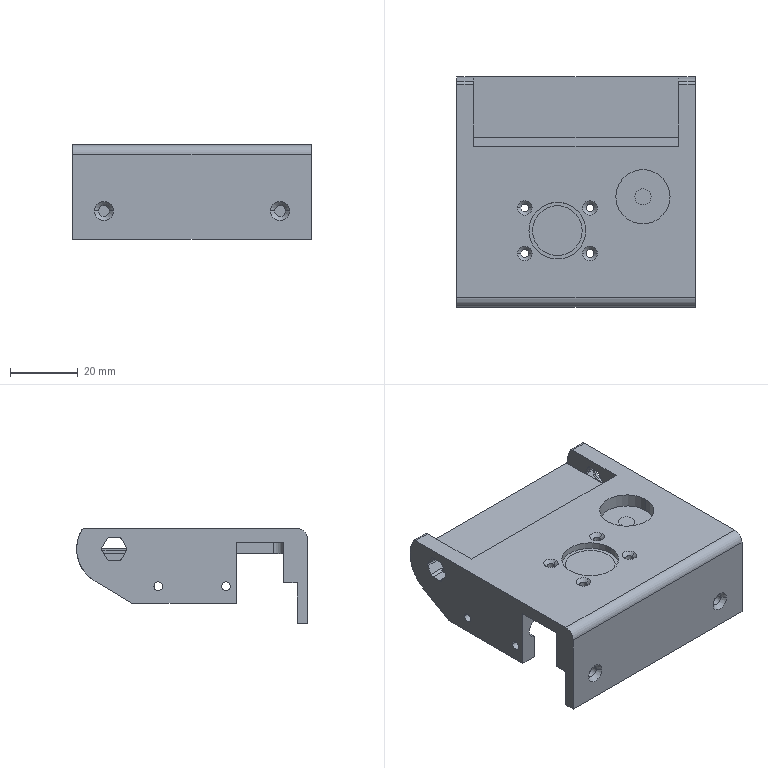NC program | NX | posted with a generic post | part box 70.5 x 68.1 x 28 mm
Lines 1 to 80 of 7250:
N10 G17 G21 G94 G90
(FLOOR_WALL_COPY , TOOL : D63)
N12 T01 M6
N14 G54
N16 G17 G0 G90 X-34.5 Y35.247 B0. C0. S6500 M3
N18 G43 Z30. H1
N20 Z9.
N22 G94 G1 Z6. F1250.
N24 X-31.5
N26 X99.6
N28 Y-10.05
N30 X-31.5
N32 X-34.5
N34 Z9.
N36 G0 Z30.
N38 Y35.247
N40 Z8.
N42 G1 Z5.
N44 X-31.5
N46 X99.6
N48 Y-10.05
N50 X-31.5
N52 X-34.5
N54 Z8.
N56 G0 Z30.
N58 Y35.247
N60 Z7.
N62 G1 Z4.
N64 X-31.5
N66 X99.6
N68 Y-10.05
N70 X-31.5
N72 X-34.5
N74 Z7.
N76 G0 Z30.
N78 Y35.247
N80 Z6.
N82 G1 Z3.
N84 X-31.5
N86 X99.6
N88 Y-10.05
N90 X-31.5
N92 X-34.5
N94 Z6.
N96 G0 Z30.
N98 Y35.247
N100 Z5.
N102 G1 Z2.
N104 X-31.5
N106 X99.6
N108 Y-10.05
N110 X-31.5
N112 X-34.5
N114 Z5.
N116 G0 Z30.
N118 Y35.247
N120 Z4.
N122 G1 Z1.
N124 X-31.5
N126 X99.6
N128 Y-10.05
N130 X-31.5
N132 X-34.5
N134 Z4.
N136 G0 Z30.
N138 Y35.247
N140 Z3.
N142 G1 Z0.
N144 X-31.5
N146 X99.6
N148 Y-10.05
N150 X-31.5
N152 X-34.5
N154 Z3.
N156 G0 Z30.
N158 M5